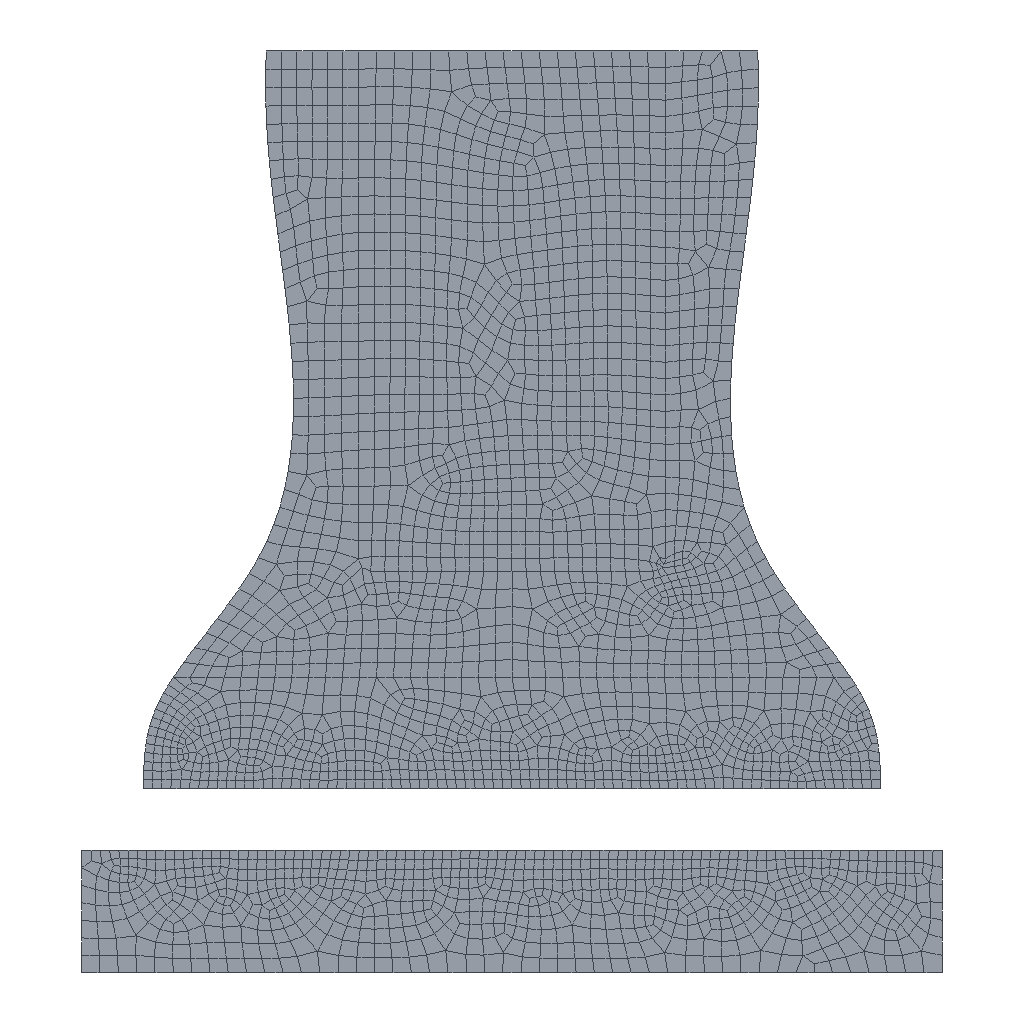Simulation study | abaqus
Set-up summary:
category,name,step,type,value,unit,region
solver,abaqus
solver,version,,,Abaqus/Standard 2020
units,not stated in the deck,,not stated
analysis,deck,,static,static
load_step,Step-1,Step-1,static
load_step,Step-3,Step-3,static
load_step,requested,,,2
mesh,nodes,,,3035
mesh,elements,,,2853
element_type,CPS4R,,plane,2853
load,load commands in deck,,count,2
bc,support commands in deck,,count,5
material,MIRROR,,in results
material,PDMS,,in results
material,SILICONRUBBER,,in results
material,TPU,,in results
check,setup vs results,,match,"per instance, exact: element labels, types and connectivity; labels of the nodes the elements use; coordinates of those nodes at SINGLE_PRECISION in 2 of 2 instance(s)"
Abaqus input file, long lists of numbers shortened:
*Heading
** Job name: Job-1 Model name: Model-1
** Generated by: Abaqus/CAE 2020
*Preprint, echo=NO, model=NO, history=NO, contact=NO
**
** PARTS
**
*Part, name=Mirror
*Node
      1,   137.021,           0.
      2,   131.064,           0.
** (843 more lines like these left out)
*Element, type=CPS4R
  1,  33,  31, 494,  72
  2,  72, 494, 455,  73
** (765 more lines like these left out)
*Nset, nset=_PickedSet3, internal, generate
   1,  845,    1
*Elset, elset=_PickedSet3, internal, generate
   1,  767,    1
*Elset, elset=_Surf-Mirror_S2, internal
  13,  19,  26,  33,  46,  60,  66,  72,  78,  84,  91,  95, 109, 115, 121, 127
 134, 141, 148, 154, 160, 164, 177, 183, 189, 195, 283, 344, 347, 349, 351, 353
** (2 more lines like these left out)
*Elset, elset=_Surf-Mirror_S4, internal
  40,  53, 102, 171, 284, 285, 287, 289, 290, 292, 293, 295, 296, 297, 299, 301
 303, 305, 307, 309, 310, 311, 313, 315, 317, 319, 321, 323, 325, 327, 329, 331
** (1 more lines like these left out)
*Elset, elset=_Surf-Mirror_S1, internal
 200, 383
*Elset, elset=_Surf-Mirror_S3, internal
 341,
*Surface, type=ELEMENT, name=Surf-Mirror
_Surf-Mirror_S2, S2
_Surf-Mirror_S4, S4
_Surf-Mirror_S1, S1
_Surf-Mirror_S3, S3
** Section: Section-mirror
*Solid Section, elset=_PickedSet3, material=Mirror
,
*End Part
**
*Part, name=mushroom
*Node
      1,           0.,  -21.88
      2,   55.12,  -21.88
** (2188 more lines like these left out)
*Element, type=CPS4R
  1, 451, 386, 376, 495
  2, 495, 493, 583, 503
** (2084 more lines like these left out)
*Nset, nset=CORE
    4,    5,    6,    7,    9,   10,   11,   73,   74,   75,   76,   77,   78,   79,   80,   81
   82,   83,   84,   85,   86,   87,   88,   89,   90,   91,   92,   93,   94,   95,   96,   97
** (45 more lines like these left out)
*Elset, elset=CORE, generate
  672,  1358,     1
*Nset, nset=SHELL
    1,    2,    3,    4,    5,    6,    7,    8,    9,   10,   11,   12,   13,   14,   15,   16
   17,   18,   19,   20,   21,   22,   23,   24,   25,   26,   27,   28,   29,   30,   31,   32
** (95 more lines like these left out)
*Elset, elset=SHELL
    1,    2,    3,    4,    5,    6,    7,    8,    9,   10,   11,   12,   13,   14,   15,   16
   17,   18,   19,   20,   21,   22,   23,   24,   25,   26,   27,   28,   29,   30,   31,   32
** (86 more lines like these left out)
*Nset, nset=TOP
   3,   4,  11,  12,  69,  70,  71,  72, 176, 177, 178, 179, 180, 216, 217, 218
 219, 220, 221, 222, 223, 224, 225, 226, 227, 228, 229, 230, 231
*Elset, elset=TOP
  54,  55, 190, 335, 344, 418, 419, 443, 445, 446, 484, 741, 742, 743, 744, 747
 748, 751, 753, 754, 755, 784, 791, 804, 808, 812, 814, 882
*Nset, nset=FORCE
 3,
*Nset, nset=BOTTOM
  13,  14, 244, 245, 246, 247, 248, 249, 250, 251, 252, 253, 254, 255, 256, 257
 258, 259, 260, 261, 262, 263, 264, 265, 266, 267, 268, 269, 270, 271, 272, 273
** (4 more lines like these left out)
*Elset, elset=BOTTOM
 1364, 1366, 1377, 1378, 1395, 1402, 1407, 1414, 1421, 1428, 1429, 1434, 1443, 1444, 1448, 1454
 1458, 1462, 1465, 1466, 1467, 1477, 1478, 1487, 1488, 1495, 1500, 1506, 1513, 1517, 1529, 1530
** (3 more lines like these left out)
*Elset, elset=_Surf-BOTTOM_S1, internal
 1364, 1366, 1377, 1378, 1395, 1407, 1421, 1434, 1443, 1448, 1454, 1458, 1462, 1465, 1466, 1467
 1477, 1478, 1487, 1488, 1495, 1500, 1506, 1513, 1517, 1660, 1685, 1691, 1694, 1696, 1697, 1699
** (1 more lines like these left out)
*Elset, elset=_Surf-BOTTOM_S3, internal
 1402, 1414, 1428, 1429, 1444, 1529, 1631, 1632, 1634, 1635, 1636, 1637, 1638, 1640, 1643, 1645
 1646, 1648, 1649, 1651, 1655, 1693, 1718, 1721, 1724, 1727, 1729, 1731, 1733, 1736, 1738, 1740
** (1 more lines like these left out)
*Elset, elset=_Surf-BOTTOM_S2, internal
 1530, 1627, 1715, 1716
*Elset, elset=_Surf-BOTTOM_S4, internal
 1659,
*Surface, type=ELEMENT, name=Surf-BOTTOM
_Surf-BOTTOM_S1, S1
_Surf-BOTTOM_S3, S3
_Surf-BOTTOM_S2, S2
_Surf-BOTTOM_S4, S4
** Section: Section-SHELL
*Solid Section, elset=SHELL, material=SiliconRubber
,
** Section: Section-CORE
*Solid Section, elset=CORE, material=SiliconRubber
,
*End Part
**
**
** ASSEMBLY
**
*Assembly, name=Assembly
**
*Instance, name=Mirror-1, part=Mirror
        -70.,         -70.,           0.
*End Instance
**
*Instance, name=mushroom-1, part=mushroom
*End Instance
**
*Node
      1,         -70.,         -50.,           0.
*Node
      2,          70.,         -50.,           0.
*Nset, nset=Set-2, instance=Mirror-1
   1,   2,   3,   4,   5,   6,   7,   8,   9,  10,  11,  12,  13,  14,  15,  16
  17,  18,  19,  20,  21,  22,  23,  24,  25,  26,  27,  28,  29,  30,  31,  32
** (1 more lines like these left out)
*Elset, elset=Set-2, instance=Mirror-1
   1,   8,   9,  15,  21,  22,  28,  35,  36,  42,  48,  49,  55,  56,  62,  68
  69,  74,  80,  86,  87,  93,  97,  98, 104, 105, 117, 123, 129, 130, 136, 143
** (1 more lines like these left out)
*Nset, nset=Set-3, instance=mushroom-1
   3,   4,  11,  12,  69,  70,  71,  72, 176, 177, 178, 179, 180, 216, 217, 218
 219, 220, 221, 222, 223, 224, 225, 226, 227, 228, 229, 230, 231
*Elset, elset=Set-3, instance=mushroom-1
  54,  55, 190, 335, 344, 418, 419, 443, 445, 446, 484, 741, 742, 743, 744, 747
 748, 751, 753, 754, 755, 784, 791, 804, 808, 812, 814, 882
*End Assembly
*Amplitude, name=Amp-1
             0.,              0.,              1.,              1.
**
** MATERIALS
**
*Material, name=Mirror
*Density
 9.3e-07,
*Elastic
10000., 0.5
*Material, name=PDMS
*Density
 9.3e-07,
*Hyperelastic, neo hooke
 0.662, 0.255
*Material, name=SiliconRubber
*Density
 9.3e-07,
*Hyperelastic, mooney-rivlin
 0.111, 0.039, 0.001
*Material, name=TPU
*Density
 9.3e-07,
*Hyperelastic, ogden
 2.54, 3.29, 0.33
**
** INTERACTION PROPERTIES
**
*Surface Interaction, name=INTPROP-1
1.,
*Friction, slip tolerance=0.005
0.,
*Surface Behavior, pressure-overclosure=HARD
*Surface Interaction, name=INTPROP-COH
1.,
*Cohesive Behavior, REPEATED CONTACTS, eligibility=CURRENT CONTACTS
 0.25, 0.25, 0.25
*Damage Initiation, criterion=MAXS
 0.05, 0.05, 0.05
*Damage Evolution, type=DISPLACEMENT, softening=EXPONENTIAL
 0.205,2.
*Damage Stabilization
0.01
**
** BOUNDARY CONDITIONS
**
** Name: BC-2 Type: 对称/反对称/完全固定
*Boundary
Set-2, ENCASTRE
**
** INTERACTIONS
**
** Interaction: Int-1
*Contact
*Contact Inclusions, ALL EXTERIOR
*Contact Property Assignment
 ,  , INTPROP-1
** ----------------------------------------------------------------
**
** STEP: Step-1
**
*Step, name=Step-1, nlgeom=YES
*Static, stabilize=0.0002, allsdtol=0.05, continue=NO
0.01, 1., 1e-05, 0.1
**
** BOUNDARY CONDITIONS
**
** Name: [REDACTED] : Displacement/rotation angle
*Boundary, amplitude=Amp-1
Set-3, 1, 1
Set-3, 2, 2, -22.9
Set-3, 6, 6
**
** OUTPUT REQUESTS
**
*Restart, write, frequency=0
**
** FIELD OUTPUT: F-Output-1
**
*Output, field
*Node Output
CF, RF, RM, RT, U, V
*Element Output, directions=YES
E, LE, MISES, MISESONLY, PE, PEEQ, PEMAG, S, SSAVG
*Contact Output
CDISP, CSTRESS
**
** HISTORY OUTPUT: H-Output-1
**
*Output, history, variable=PRESELECT
*End Step
** ----------------------------------------------------------------
**
** STEP: Step-3
**
*Step, name=Step-3, nlgeom=YES, inc=10000000
*Static, stabilize=0.0002, allsdtol=0.05, continue=NO
0.001, 1., 1e-10, 0.01
**
** BOUNDARY CONDITIONS
**
** Name: [REDACTED] : Displacement/rotation angle
*Boundary, amplitude=Amp-1
Set-3, 2, 2, 30.
**
** OUTPUT REQUESTS
**
*Restart, write, frequency=0
**
** FIELD OUTPUT: F-Output-1
**
*Output, field
*Node Output
CF, RF, RM, RT, U, V
*Element Output, directions=YES
E, LE, MISES, MISESONLY, PE, PEEQ, PEMAG, S, SSAVG
*Contact Output
CDISP, CSTRESS
**
** HISTORY OUTPUT: H-Output-1
**
*Output, history, variable=PRESELECT
*End Step
Results summary:
result,step,,completed,increments=16 time=1.0/1.0
result,step,,completed,increments=120 time=1.0/1.0
result,analysis,,,static
result,last_loadstep,,,2
result,primary field,,,U
result,reaction total,,FX,-0.0,model units
result,reaction total,,FY,0.0,model units
result,reaction total,,FZ,0.0,model units